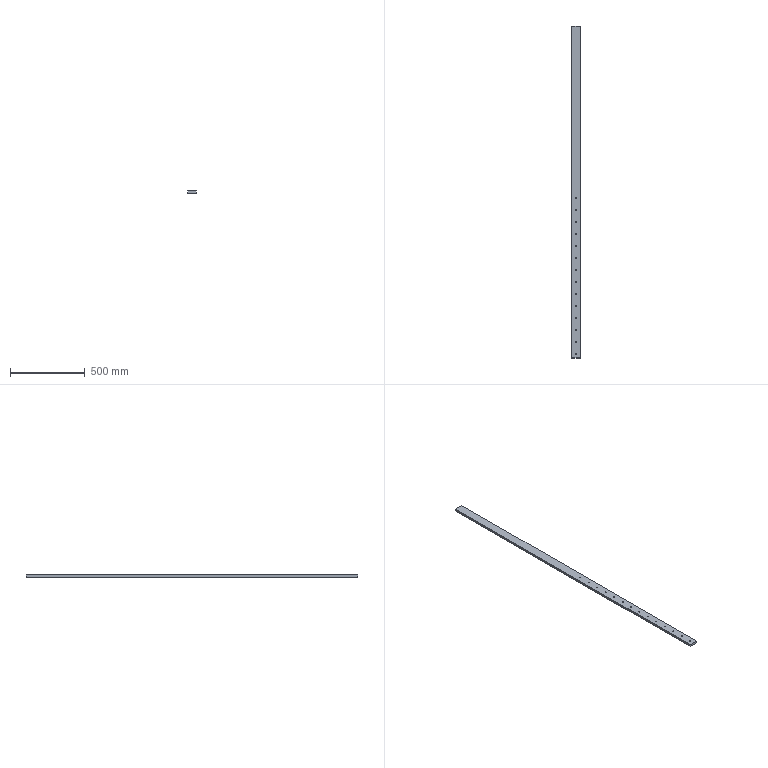Part | SolidWorks | features BaseBody 1 | 1 solid | 34 faces | box 60 x 2220 x 15 mm | volume 1990373 mm3 | cylinder 28 | plane 6 | commonest cylinder face diameters 6.8 x28
STEP:
#1=CARTESIAN_POINT('',(563.4,1142.,-1300.));
#2=VERTEX_POINT('',#1);
#3=CARTESIAN_POINT('',(556.6,1142.,-1300.));
#4=VERTEX_POINT('',#3);
#5=CARTESIAN_POINT('',(560.,1142.,-1300.));
#6=DIRECTION('',(0.,0.,-1.));
#7=DIRECTION('',(1.,0.,0.));
#8=AXIS2_PLACEMENT_3D('',#5,#6,#7);
#9=CIRCLE('',#8,3.4);
#10=EDGE_CURVE('',#2,#4,#9,.T.);
#11=ORIENTED_EDGE('',*,*,#10,.T.);
#12=CARTESIAN_POINT('',(556.6,1142.,-1285.));
#13=VERTEX_POINT('',#12);
#14=CARTESIAN_POINT('',(556.6,1142.,-1285.));
#15=DIRECTION('',(0.,0.,1.));
#16=VECTOR('',#15,1000.);
#17=LINE('',#14,#16);
#18=EDGE_CURVE('',#4,#13,#17,.T.);
#19=ORIENTED_EDGE('',*,*,#18,.T.);
#20=CARTESIAN_POINT('',(563.4,1142.,-1285.));
#21=VERTEX_POINT('',#20);
#22=CARTESIAN_POINT('',(560.,1142.,-1285.));
#23=DIRECTION('',(0.,0.,-1.));
#24=DIRECTION('',(1.,0.,0.));
#25=AXIS2_PLACEMENT_3D('',#22,#23,#24);
#26=CIRCLE('',#25,3.4);
#27=EDGE_CURVE('',#21,#13,#26,.T.);
#28=ORIENTED_EDGE('',*,*,#27,.F.);
#29=CARTESIAN_POINT('',(563.4,1142.,-1285.));
#30=DIRECTION('',(0.,0.,1.));
#31=VECTOR('',#30,1000.);
#32=LINE('',#29,#31);
#33=EDGE_CURVE('',#2,#21,#32,.T.);
#34=ORIENTED_EDGE('',*,*,#33,.F.);
#35=EDGE_LOOP('',(#11,#19,#28,#34));
#36=FACE_OUTER_BOUND('',#35,.T.);
#37=CARTESIAN_POINT('',(560.,1142.,-1285.));
#38=DIRECTION('',(0.,0.,1.));
#39=DIRECTION('',(1.,0.,0.));
#40=AXIS2_PLACEMENT_3D('',#37,#38,#39);
#41=CYLINDRICAL_SURFACE('',#40,3.4);
#42=ADVANCED_FACE('',(#36),#41,.F.);
#43=CARTESIAN_POINT('',(563.4,102.,-1300.));
#44=VERTEX_POINT('',#43);
#45=CARTESIAN_POINT('',(556.6,102.,-1300.));
#46=VERTEX_POINT('',#45);
#47=CARTESIAN_POINT('',(560.,102.,-1300.));
#48=DIRECTION('',(0.,0.,-1.));
#49=DIRECTION('',(1.,0.,0.));
#50=AXIS2_PLACEMENT_3D('',#47,#48,#49);
#51=CIRCLE('',#50,3.4);
#52=EDGE_CURVE('',#44,#46,#51,.T.);
#53=ORIENTED_EDGE('',*,*,#52,.T.);
#54=CARTESIAN_POINT('',(556.6,102.,-1285.));
#55=VERTEX_POINT('',#54);
#56=CARTESIAN_POINT('',(556.6,102.,-1285.));
#57=DIRECTION('',(0.,0.,1.));
#58=VECTOR('',#57,1000.);
#59=LINE('',#56,#58);
#60=EDGE_CURVE('',#46,#55,#59,.T.);
#61=ORIENTED_EDGE('',*,*,#60,.T.);
#62=CARTESIAN_POINT('',(563.4,102.,-1285.));
#63=VERTEX_POINT('',#62);
#64=CARTESIAN_POINT('',(560.,102.,-1285.));
#65=DIRECTION('',(0.,0.,-1.));
#66=DIRECTION('',(1.,0.,0.));
#67=AXIS2_PLACEMENT_3D('',#64,#65,#66);
#68=CIRCLE('',#67,3.4);
#69=EDGE_CURVE('',#63,#55,#68,.T.);
#70=ORIENTED_EDGE('',*,*,#69,.F.);
#71=CARTESIAN_POINT('',(563.4,102.,-1285.));
#72=DIRECTION('',(0.,0.,1.));
#73=VECTOR('',#72,1000.);
#74=LINE('',#71,#73);
#75=EDGE_CURVE('',#44,#63,#74,.T.);
#76=ORIENTED_EDGE('',*,*,#75,.F.);
#77=EDGE_LOOP('',(#53,#61,#70,#76));
#78=FACE_OUTER_BOUND('',#77,.T.);
#79=CARTESIAN_POINT('',(560.,102.,-1285.));
#80=DIRECTION('',(0.,0.,1.));
#81=DIRECTION('',(1.,0.,0.));
#82=AXIS2_PLACEMENT_3D('',#79,#80,#81);
#83=CYLINDRICAL_SURFACE('',#82,3.4);
#84=ADVANCED_FACE('',(#78),#83,.F.);
#85=CARTESIAN_POINT('',(563.4,182.,-1300.));
#86=VERTEX_POINT('',#85);
#87=CARTESIAN_POINT('',(556.6,182.,-1300.));
#88=VERTEX_POINT('',#87);
#89=CARTESIAN_POINT('',(560.,182.,-1300.));
#90=DIRECTION('',(0.,0.,-1.));
#91=DIRECTION('',(1.,0.,0.));
#92=AXIS2_PLACEMENT_3D('',#89,#90,#91);
#93=CIRCLE('',#92,3.4);
#94=EDGE_CURVE('',#86,#88,#93,.T.);
#95=ORIENTED_EDGE('',*,*,#94,.T.);
#96=CARTESIAN_POINT('',(556.6,182.,-1285.));
#97=VERTEX_POINT('',#96);
#98=CARTESIAN_POINT('',(556.6,182.,-1285.));
#99=DIRECTION('',(0.,0.,1.));
#100=VECTOR('',#99,1000.);
#101=LINE('',#98,#100);
#102=EDGE_CURVE('',#88,#97,#101,.T.);
#103=ORIENTED_EDGE('',*,*,#102,.T.);
#104=CARTESIAN_POINT('',(563.4,182.,-1285.));
#105=VERTEX_POINT('',#104);
#106=CARTESIAN_POINT('',(560.,182.,-1285.));
#107=DIRECTION('',(0.,0.,-1.));
#108=DIRECTION('',(1.,0.,0.));
#109=AXIS2_PLACEMENT_3D('',#106,#107,#108);
#110=CIRCLE('',#109,3.4);
#111=EDGE_CURVE('',#105,#97,#110,.T.);
#112=ORIENTED_EDGE('',*,*,#111,.F.);
#113=CARTESIAN_POINT('',(563.4,182.,-1285.));
#114=DIRECTION('',(0.,0.,1.));
#115=VECTOR('',#114,1000.);
#116=LINE('',#113,#115);
#117=EDGE_CURVE('',#86,#105,#116,.T.);
#118=ORIENTED_EDGE('',*,*,#117,.F.);
#119=EDGE_LOOP('',(#95,#103,#112,#118));
#120=FACE_OUTER_BOUND('',#119,.T.);
#121=CARTESIAN_POINT('',(560.,182.,-1285.));
#122=DIRECTION('',(0.,0.,1.));
#123=DIRECTION('',(1.,0.,0.));
#124=AXIS2_PLACEMENT_3D('',#121,#122,#123);
#125=CYLINDRICAL_SURFACE('',#124,3.4);
#126=ADVANCED_FACE('',(#120),#125,.F.);
#127=CARTESIAN_POINT('',(563.4,262.,-1300.));
#128=VERTEX_POINT('',#127);
#129=CARTESIAN_POINT('',(556.6,262.,-1300.));
#130=VERTEX_POINT('',#129);
#131=CARTESIAN_POINT('',(560.,262.,-1300.));
#132=DIRECTION('',(0.,0.,-1.));
#133=DIRECTION('',(1.,0.,0.));
#134=AXIS2_PLACEMENT_3D('',#131,#132,#133);
#135=CIRCLE('',#134,3.4);
#136=EDGE_CURVE('',#128,#130,#135,.T.);
#137=ORIENTED_EDGE('',*,*,#136,.T.);
#138=CARTESIAN_POINT('',(556.6,262.,-1285.));
#139=VERTEX_POINT('',#138);
#140=CARTESIAN_POINT('',(556.6,262.,-1285.));
#141=DIRECTION('',(0.,0.,1.));
#142=VECTOR('',#141,1000.);
#143=LINE('',#140,#142);
#144=EDGE_CURVE('',#130,#139,#143,.T.);
#145=ORIENTED_EDGE('',*,*,#144,.T.);
#146=CARTESIAN_POINT('',(563.4,262.,-1285.));
#147=VERTEX_POINT('',#146);
#148=CARTESIAN_POINT('',(560.,262.,-1285.));
#149=DIRECTION('',(0.,0.,-1.));
#150=DIRECTION('',(1.,0.,0.));
#151=AXIS2_PLACEMENT_3D('',#148,#149,#150);
#152=CIRCLE('',#151,3.4);
#153=EDGE_CURVE('',#147,#139,#152,.T.);
#154=ORIENTED_EDGE('',*,*,#153,.F.);
#155=CARTESIAN_POINT('',(563.4,262.,-1285.));
#156=DIRECTION('',(0.,0.,1.));
#157=VECTOR('',#156,1000.);
#158=LINE('',#155,#157);
#159=EDGE_CURVE('',#128,#147,#158,.T.);
#160=ORIENTED_EDGE('',*,*,#159,.F.);
#161=EDGE_LOOP('',(#137,#145,#154,#160));
#162=FACE_OUTER_BOUND('',#161,.T.);
#163=CARTESIAN_POINT('',(560.,262.,-1285.));
#164=DIRECTION('',(0.,0.,1.));
#165=DIRECTION('',(1.,0.,0.));
#166=AXIS2_PLACEMENT_3D('',#163,#164,#165);
#167=CYLINDRICAL_SURFACE('',#166,3.4);
#168=ADVANCED_FACE('',(#162),#167,.F.);
#169=CARTESIAN_POINT('',(563.4,342.,-1300.));
#170=VERTEX_POINT('',#169);
#171=CARTESIAN_POINT('',(556.6,342.,-1300.));
#172=VERTEX_POINT('',#171);
#173=CARTESIAN_POINT('',(560.,342.,-1300.));
#174=DIRECTION('',(0.,0.,-1.));
#175=DIRECTION('',(1.,0.,0.));
#176=AXIS2_PLACEMENT_3D('',#173,#174,#175);
#177=CIRCLE('',#176,3.4);
#178=EDGE_CURVE('',#170,#172,#177,.T.);
#179=ORIENTED_EDGE('',*,*,#178,.T.);
#180=CARTESIAN_POINT('',(556.6,342.,-1285.));
#181=VERTEX_POINT('',#180);
#182=CARTESIAN_POINT('',(556.6,342.,-1285.));
#183=DIRECTION('',(0.,0.,1.));
#184=VECTOR('',#183,1000.);
#185=LINE('',#182,#184);
#186=EDGE_CURVE('',#172,#181,#185,.T.);
#187=ORIENTED_EDGE('',*,*,#186,.T.);
#188=CARTESIAN_POINT('',(563.4,342.,-1285.));
#189=VERTEX_POINT('',#188);
#190=CARTESIAN_POINT('',(560.,342.,-1285.));
#191=DIRECTION('',(0.,0.,-1.));
#192=DIRECTION('',(1.,0.,0.));
#193=AXIS2_PLACEMENT_3D('',#190,#191,#192);
#194=CIRCLE('',#193,3.4);
#195=EDGE_CURVE('',#189,#181,#194,.T.);
#196=ORIENTED_EDGE('',*,*,#195,.F.);
#197=CARTESIAN_POINT('',(563.4,342.,-1285.));
#198=DIRECTION('',(0.,0.,1.));
#199=VECTOR('',#198,1000.);
#200=LINE('',#197,#199);
#201=EDGE_CURVE('',#170,#189,#200,.T.);
#202=ORIENTED_EDGE('',*,*,#201,.F.);
#203=EDGE_LOOP('',(#179,#187,#196,#202));
#204=FACE_OUTER_BOUND('',#203,.T.);
#205=CARTESIAN_POINT('',(560.,342.,-1285.));
#206=DIRECTION('',(0.,0.,1.));
#207=DIRECTION('',(1.,0.,0.));
#208=AXIS2_PLACEMENT_3D('',#205,#206,#207);
#209=CYLINDRICAL_SURFACE('',#208,3.4);
#210=ADVANCED_FACE('',(#204),#209,.F.);
#211=CARTESIAN_POINT('',(563.4,422.,-1300.));
#212=VERTEX_POINT('',#211);
#213=CARTESIAN_POINT('',(556.6,422.,-1300.));
#214=VERTEX_POINT('',#213);
#215=CARTESIAN_POINT('',(560.,422.,-1300.));
#216=DIRECTION('',(0.,0.,-1.));
#217=DIRECTION('',(1.,0.,0.));
#218=AXIS2_PLACEMENT_3D('',#215,#216,#217);
#219=CIRCLE('',#218,3.4);
#220=EDGE_CURVE('',#212,#214,#219,.T.);
#221=ORIENTED_EDGE('',*,*,#220,.T.);
#222=CARTESIAN_POINT('',(556.6,422.,-1285.));
#223=VERTEX_POINT('',#222);
#224=CARTESIAN_POINT('',(556.6,422.,-1285.));
#225=DIRECTION('',(0.,0.,1.));
#226=VECTOR('',#225,1000.);
#227=LINE('',#224,#226);
#228=EDGE_CURVE('',#214,#223,#227,.T.);
#229=ORIENTED_EDGE('',*,*,#228,.T.);
#230=CARTESIAN_POINT('',(563.4,422.,-1285.));
#231=VERTEX_POINT('',#230);
#232=CARTESIAN_POINT('',(560.,422.,-1285.));
#233=DIRECTION('',(0.,0.,-1.));
#234=DIRECTION('',(1.,0.,0.));
#235=AXIS2_PLACEMENT_3D('',#232,#233,#234);
#236=CIRCLE('',#235,3.4);
#237=EDGE_CURVE('',#231,#223,#236,.T.);
#238=ORIENTED_EDGE('',*,*,#237,.F.);
#239=CARTESIAN_POINT('',(563.4,422.,-1285.));
#240=DIRECTION('',(0.,0.,1.));
#241=VECTOR('',#240,1000.);
#242=LINE('',#239,#241);
#243=EDGE_CURVE('',#212,#231,#242,.T.);
#244=ORIENTED_EDGE('',*,*,#243,.F.);
#245=EDGE_LOOP('',(#221,#229,#238,#244));
#246=FACE_OUTER_BOUND('',#245,.T.);
#247=CARTESIAN_POINT('',(560.,422.,-1285.));
#248=DIRECTION('',(0.,0.,1.));
#249=DIRECTION('',(1.,0.,0.));
#250=AXIS2_PLACEMENT_3D('',#247,#248,#249);
#251=CYLINDRICAL_SURFACE('',#250,3.4);
#252=ADVANCED_FACE('',(#246),#251,.F.);
#253=CARTESIAN_POINT('',(563.4,502.,-1300.));
#254=VERTEX_POINT('',#253);
#255=CARTESIAN_POINT('',(556.6,502.,-1300.));
#256=VERTEX_POINT('',#255);
#257=CARTESIAN_POINT('',(560.,502.,-1300.));
#258=DIRECTION('',(0.,0.,-1.));
#259=DIRECTION('',(1.,0.,0.));
#260=AXIS2_PLACEMENT_3D('',#257,#258,#259);
#261=CIRCLE('',#260,3.4);
#262=EDGE_CURVE('',#254,#256,#261,.T.);
#263=ORIENTED_EDGE('',*,*,#262,.T.);
#264=CARTESIAN_POINT('',(556.6,502.,-1285.));
#265=VERTEX_POINT('',#264);
#266=CARTESIAN_POINT('',(556.6,502.,-1285.));
#267=DIRECTION('',(0.,0.,1.));
#268=VECTOR('',#267,1000.);
#269=LINE('',#266,#268);
#270=EDGE_CURVE('',#256,#265,#269,.T.);
#271=ORIENTED_EDGE('',*,*,#270,.T.);
#272=CARTESIAN_POINT('',(563.4,502.,-1285.));
#273=VERTEX_POINT('',#272);
#274=CARTESIAN_POINT('',(560.,502.,-1285.));
#275=DIRECTION('',(0.,0.,-1.));
#276=DIRECTION('',(1.,0.,0.));
#277=AXIS2_PLACEMENT_3D('',#274,#275,#276);
#278=CIRCLE('',#277,3.4);
#279=EDGE_CURVE('',#273,#265,#278,.T.);
#280=ORIENTED_EDGE('',*,*,#279,.F.);
#281=CARTESIAN_POINT('',(563.4,502.,-1285.));
#282=DIRECTION('',(0.,0.,1.));
#283=VECTOR('',#282,1000.);
#284=LINE('',#281,#283);
#285=EDGE_CURVE('',#254,#273,#284,.T.);
#286=ORIENTED_EDGE('',*,*,#285,.F.);
#287=EDGE_LOOP('',(#263,#271,#280,#286));
#288=FACE_OUTER_BOUND('',#287,.T.);
#289=CARTESIAN_POINT('',(560.,502.,-1285.));
#290=DIRECTION('',(0.,0.,1.));
#291=DIRECTION('',(1.,0.,0.));
#292=AXIS2_PLACEMENT_3D('',#289,#290,#291);
#293=CYLINDRICAL_SURFACE('',#292,3.4);
#294=ADVANCED_FACE('',(#288),#293,.F.);
#295=CARTESIAN_POINT('',(563.4,582.,-1300.));
#296=VERTEX_POINT('',#295);
#297=CARTESIAN_POINT('',(556.6,582.,-1300.));
#298=VERTEX_POINT('',#297);
#299=CARTESIAN_POINT('',(560.,582.,-1300.));
#300=DIRECTION('',(0.,0.,-1.));
#301=DIRECTION('',(1.,0.,0.));
#302=AXIS2_PLACEMENT_3D('',#299,#300,#301);
#303=CIRCLE('',#302,3.4);
#304=EDGE_CURVE('',#296,#298,#303,.T.);
#305=ORIENTED_EDGE('',*,*,#304,.T.);
#306=CARTESIAN_POINT('',(556.6,582.,-1285.));
#307=VERTEX_POINT('',#306);
#308=CARTESIAN_POINT('',(556.6,582.,-1285.));
#309=DIRECTION('',(0.,0.,1.));
#310=VECTOR('',#309,1000.);
#311=LINE('',#308,#310);
#312=EDGE_CURVE('',#298,#307,#311,.T.);
#313=ORIENTED_EDGE('',*,*,#312,.T.);
#314=CARTESIAN_POINT('',(563.4,582.,-1285.));
#315=VERTEX_POINT('',#314);
#316=CARTESIAN_POINT('',(560.,582.,-1285.));
#317=DIRECTION('',(0.,0.,-1.));
#318=DIRECTION('',(1.,0.,0.));
#319=AXIS2_PLACEMENT_3D('',#316,#317,#318);
#320=CIRCLE('',#319,3.4);
#321=EDGE_CURVE('',#315,#307,#320,.T.);
#322=ORIENTED_EDGE('',*,*,#321,.F.);
#323=CARTESIAN_POINT('',(563.4,582.,-1285.));
#324=DIRECTION('',(0.,0.,1.));
#325=VECTOR('',#324,1000.);
#326=LINE('',#323,#325);
#327=EDGE_CURVE('',#296,#315,#326,.T.);
#328=ORIENTED_EDGE('',*,*,#327,.F.);
#329=EDGE_LOOP('',(#305,#313,#322,#328));
#330=FACE_OUTER_BOUND('',#329,.T.);
#331=CARTESIAN_POINT('',(560.,582.,-1285.));
#332=DIRECTION('',(0.,0.,1.));
#333=DIRECTION('',(1.,0.,0.));
#334=AXIS2_PLACEMENT_3D('',#331,#332,#333);
#335=CYLINDRICAL_SURFACE('',#334,3.4);
#336=ADVANCED_FACE('',(#330),#335,.F.);
#337=CARTESIAN_POINT('',(563.4,662.,-1300.));
#338=VERTEX_POINT('',#337);
#339=CARTESIAN_POINT('',(556.6,662.,-1300.));
#340=VERTEX_POINT('',#339);
#341=CARTESIAN_POINT('',(560.,662.,-1300.));
#342=DIRECTION('',(0.,0.,-1.));
#343=DIRECTION('',(1.,0.,0.));
#344=AXIS2_PLACEMENT_3D('',#341,#342,#343);
#345=CIRCLE('',#344,3.4);
#346=EDGE_CURVE('',#338,#340,#345,.T.);
#347=ORIENTED_EDGE('',*,*,#346,.T.);
#348=CARTESIAN_POINT('',(556.6,662.,-1285.));
#349=VERTEX_POINT('',#348);
#350=CARTESIAN_POINT('',(556.6,662.,-1285.));
#351=DIRECTION('',(0.,0.,1.));
#352=VECTOR('',#351,1000.);
#353=LINE('',#350,#352);
#354=EDGE_CURVE('',#340,#349,#353,.T.);
#355=ORIENTED_EDGE('',*,*,#354,.T.);
#356=CARTESIAN_POINT('',(563.4,662.,-1285.));
#357=VERTEX_POINT('',#356);
#358=CARTESIAN_POINT('',(560.,662.,-1285.));
#359=DIRECTION('',(0.,0.,-1.));
#360=DIRECTION('',(1.,0.,0.));
#361=AXIS2_PLACEMENT_3D('',#358,#359,#360);
#362=CIRCLE('',#361,3.4);
#363=EDGE_CURVE('',#357,#349,#362,.T.);
#364=ORIENTED_EDGE('',*,*,#363,.F.);
#365=CARTESIAN_POINT('',(563.4,662.,-1285.));
#366=DIRECTION('',(0.,0.,1.));
#367=VECTOR('',#366,1000.);
#368=LINE('',#365,#367);
#369=EDGE_CURVE('',#338,#357,#368,.T.);
#370=ORIENTED_EDGE('',*,*,#369,.F.);
#371=EDGE_LOOP('',(#347,#355,#364,#370));
#372=FACE_OUTER_BOUND('',#371,.T.);
#373=CARTESIAN_POINT('',(560.,662.,-1285.));
#374=DIRECTION('',(0.,0.,1.));
#375=DIRECTION('',(1.,0.,0.));
#376=AXIS2_PLACEMENT_3D('',#373,#374,#375);
#377=CYLINDRICAL_SURFACE('',#376,3.4);
#378=ADVANCED_FACE('',(#372),#377,.F.);
#379=CARTESIAN_POINT('',(563.4,742.,-1300.));
#380=VERTEX_POINT('',#379);
#381=CARTESIAN_POINT('',(556.6,742.,-1300.));
#382=VERTEX_POINT('',#381);
#383=CARTESIAN_POINT('',(560.,742.,-1300.));
#384=DIRECTION('',(0.,0.,-1.));
#385=DIRECTION('',(1.,0.,0.));
#386=AXIS2_PLACEMENT_3D('',#383,#384,#385);
#387=CIRCLE('',#386,3.4);
#388=EDGE_CURVE('',#380,#382,#387,.T.);
#389=ORIENTED_EDGE('',*,*,#388,.T.);
#390=CARTESIAN_POINT('',(556.6,742.,-1285.));
#391=VERTEX_POINT('',#390);
#392=CARTESIAN_POINT('',(556.6,742.,-1285.));
#393=DIRECTION('',(0.,0.,1.));
#394=VECTOR('',#393,1000.);
#395=LINE('',#392,#394);
#396=EDGE_CURVE('',#382,#391,#395,.T.);
#397=ORIENTED_EDGE('',*,*,#396,.T.);
#398=CARTESIAN_POINT('',(563.4,742.,-1285.));
#399=VERTEX_POINT('',#398);
#400=CARTESIAN_POINT('',(560.,742.,-1285.));
#401=DIRECTION('',(0.,0.,-1.));
#402=DIRECTION('',(1.,0.,0.));
#403=AXIS2_PLACEMENT_3D('',#400,#401,#402);
#404=CIRCLE('',#403,3.4);
#405=EDGE_CURVE('',#399,#391,#404,.T.);
#406=ORIENTED_EDGE('',*,*,#405,.F.);
#407=CARTESIAN_POINT('',(563.4,742.,-1285.));
#408=DIRECTION('',(0.,0.,1.));
#409=VECTOR('',#408,1000.);
#410=LINE('',#407,#409);
#411=EDGE_CURVE('',#380,#399,#410,.T.);
#412=ORIENTED_EDGE('',*,*,#411,.F.);
#413=EDGE_LOOP('',(#389,#397,#406,#412));
#414=FACE_OUTER_BOUND('',#413,.T.);
#415=CARTESIAN_POINT('',(560.,742.,-1285.));
#416=DIRECTION('',(0.,0.,1.));
#417=DIRECTION('',(1.,0.,0.));
#418=AXIS2_PLACEMENT_3D('',#415,#416,#417);
#419=CYLINDRICAL_SURFACE('',#418,3.4);
#420=ADVANCED_FACE('',(#414),#419,.F.);
#421=CARTESIAN_POINT('',(563.4,822.,-1300.));
#422=VERTEX_POINT('',#421);
#423=CARTESIAN_POINT('',(556.6,822.,-1300.));
#424=VERTEX_POINT('',#423);
#425=CARTESIAN_POINT('',(560.,822.,-1300.));
#426=DIRECTION('',(0.,0.,-1.));
#427=DIRECTION('',(1.,0.,0.));
#428=AXIS2_PLACEMENT_3D('',#425,#426,#427);
#429=CIRCLE('',#428,3.4);
#430=EDGE_CURVE('',#422,#424,#429,.T.);
#431=ORIENTED_EDGE('',*,*,#430,.T.);
#432=CARTESIAN_POINT('',(556.6,822.,-1285.));
#433=VERTEX_POINT('',#432);
#434=CARTESIAN_POINT('',(556.6,822.,-1285.));
#435=DIRECTION('',(0.,0.,1.));
#436=VECTOR('',#435,1000.);
#437=LINE('',#434,#436);
#438=EDGE_CURVE('',#424,#433,#437,.T.);
#439=ORIENTED_EDGE('',*,*,#438,.T.);
#440=CARTESIAN_POINT('',(563.4,822.,-1285.));
#441=VERTEX_POINT('',#440);
#442=CARTESIAN_POINT('',(560.,822.,-1285.));
#443=DIRECTION('',(0.,0.,-1.));
#444=DIRECTION('',(1.,0.,0.));
#445=AXIS2_PLACEMENT_3D('',#442,#443,#444);
#446=CIRCLE('',#445,3.4);
#447=EDGE_CURVE('',#441,#433,#446,.T.);
#448=ORIENTED_EDGE('',*,*,#447,.F.);
#449=CARTESIAN_POINT('',(563.4,822.,-1285.));
#450=DIRECTION('',(0.,0.,1.));
#451=VECTOR('',#450,1000.);
#452=LINE('',#449,#451);
#453=EDGE_CURVE('',#422,#441,#452,.T.);
#454=ORIENTED_EDGE('',*,*,#453,.F.);
#455=EDGE_LOOP('',(#431,#439,#448,#454));
#456=FACE_OUTER_BOUND('',#455,.T.);
#457=CARTESIAN_POINT('',(560.,822.,-1285.));
#458=DIRECTION('',(0.,0.,1.));
#459=DIRECTION('',(1.,0.,0.));
#460=AXIS2_PLACEMENT_3D('',#457,#458,#459);
#461=CYLINDRICAL_SURFACE('',#460,3.4);
#462=ADVANCED_FACE('',(#456),#461,.F.);
#463=CARTESIAN_POINT('',(563.4,902.,-1300.));
#464=VERTEX_POINT('',#463);
#465=CARTESIAN_POINT('',(556.6,902.,-1300.));
#466=VERTEX_POINT('',#465);
#467=CARTESIAN_POINT('',(560.,902.,-1300.));
#468=DIRECTION('',(0.,0.,-1.));
#469=DIRECTION('',(1.,0.,0.));
#470=AXIS2_PLACEMENT_3D('',#467,#468,#469);
#471=CIRCLE('',#470,3.4);
#472=EDGE_CURVE('',#464,#466,#471,.T.);
#473=ORIENTED_EDGE('',*,*,#472,.T.);
#474=CARTESIAN_POINT('',(556.6,902.,-1285.));
#475=VERTEX_POINT('',#474);
#476=CARTESIAN_POINT('',(556.6,902.,-1285.));
#477=DIRECTION('',(0.,0.,1.));
#478=VECTOR('',#477,1000.);
#479=LINE('',#476,#478);
#480=EDGE_CURVE('',#466,#475,#479,.T.);
#481=ORIENTED_EDGE('',*,*,#480,.T.);
#482=CARTESIAN_POINT('',(563.4,902.,-1285.));
#483=VERTEX_POINT('',#482);
#484=CARTESIAN_POINT('',(560.,902.,-1285.));
#485=DIRECTION('',(0.,0.,-1.));
#486=DIRECTION('',(1.,0.,0.));
#487=AXIS2_PLACEMENT_3D('',#484,#485,#486);
#488=CIRCLE('',#487,3.4);
#489=EDGE_CURVE('',#483,#475,#488,.T.);
#490=ORIENTED_EDGE('',*,*,#489,.F.);
#491=CARTESIAN_POINT('',(563.4,902.,-1285.));
#492=DIRECTION('',(0.,0.,1.));
#493=VECTOR('',#492,1000.);
#494=LINE('',#491,#493);
#495=EDGE_CURVE('',#464,#483,#494,.T.);
#496=ORIENTED_EDGE('',*,*,#495,.F.);
#497=EDGE_LOOP('',(#473,#481,#490,#496));
#498=FACE_OUTER_BOUND('',#497,.T.);
#499=CARTESIAN_POINT('',(560.,902.,-1285.));
#500=DIRECTION('',(0.,0.,1.));
#501=DIRECTION('',(1.,0.,0.));
#502=AXIS2_PLACEMENT_3D('',#499,#500,#501);
#503=CYLINDRICAL_SURFACE('',#502,3.4);
#504=ADVANCED_FACE('',(#498),#503,.F.);
#505=CARTESIAN_POINT('',(563.4,982.,-1300.));
#506=VERTEX_POINT('',#505);
#507=CARTESIAN_POINT('',(556.6,982.,-1300.));
#508=VERTEX_POINT('',#507);
#509=CARTESIAN_POINT('',(560.,982.,-1300.));
#510=DIRECTION('',(0.,0.,-1.));
#511=DIRECTION('',(1.,0.,0.));
#512=AXIS2_PLACEMENT_3D('',#509,#510,#511);
#513=CIRCLE('',#512,3.4);
#514=EDGE_CURVE('',#506,#508,#513,.T.);
#515=ORIENTED_EDGE('',*,*,#514,.T.);
#516=CARTESIAN_POINT('',(556.6,982.,-1285.));
#517=VERTEX_POINT('',#516);
#518=CARTESIAN_POINT('',(556.6,982.,-1285.));
#519=DIRECTION('',(0.,0.,1.));
#520=VECTOR('',#519,1000.);
#521=LINE('',#518,#520);
#522=EDGE_CURVE('',#508,#517,#521,.T.);
#523=ORIENTED_EDGE('',*,*,#522,.T.);
#524=CARTESIAN_POINT('',(563.4,982.,-1285.));
#525=VERTEX_POINT('',#524);
#526=CARTESIAN_POINT('',(560.,982.,-1285.));
#527=DIRECTION('',(0.,0.,-1.));
#528=DIRECTION('',(1.,0.,0.));
#529=AXIS2_PLACEMENT_3D('',#526,#527,#528);
#530=CIRCLE('',#529,3.4);
#531=EDGE_CURVE('',#525,#517,#530,.T.);
#532=ORIENTED_EDGE('',*,*,#531,.F.);
#533=CARTESIAN_POINT('',(563.4,982.,-1285.));
#534=DIRECTION('',(0.,0.,1.));
#535=VECTOR('',#534,1000.);
#536=LINE('',#533,#535);
#537=EDGE_CURVE('',#506,#525,#536,.T.);
#538=ORIENTED_EDGE('',*,*,#537,.F.);
#539=EDGE_LOOP('',(#515,#523,#532,#538));
#540=FACE_OUTER_BOUND('',#539,.T.);
#541=CARTESIAN_POINT('',(560.,982.,-1285.));
#542=DIRECTION('',(0.,0.,1.));
#543=DIRECTION('',(1.,0.,0.));
#544=AXIS2_PLACEMENT_3D('',#541,#542,#543);
#545=CYLINDRICAL_SURFACE('',#544,3.4);
#546=ADVANCED_FACE('',(#540),#545,.F.);
#547=CARTESIAN_POINT('',(563.4,1062.,-1300.));
#548=VERTEX_POINT('',#547);
#549=CARTESIAN_POINT('',(556.6,1062.,-1300.));
#550=VERTEX_POINT('',#549);
#551=CARTESIAN_POINT('',(560.,1062.,-1300.));
#552=DIRECTION('',(0.,0.,-1.));
#553=DIRECTION('',(1.,0.,0.));
#554=AXIS2_PLACEMENT_3D('',#551,#552,#553);
#555=CIRCLE('',#554,3.4);
#556=EDGE_CURVE('',#548,#550,#555,.T.);
#557=ORIENTED_EDGE('',*,*,#556,.T.);
#558=CARTESIAN_POINT('',(556.6,1062.,-1285.));
#559=VERTEX_POINT('',#558);
#560=CARTESIAN_POINT('',(556.6,1062.,-1285.));
#561=DIRECTION('',(0.,0.,1.));
#562=VECTOR('',#561,1000.);
#563=LINE('',#560,#562);
#564=EDGE_CURVE('',#550,#559,#563,.T.);
#565=ORIENTED_EDGE('',*,*,#564,.T.);
#566=CARTESIAN_POINT('',(563.4,1062.,-1285.));
#567=VERTEX_POINT('',#566);
#568=CARTESIAN_POINT('',(560.,1062.,-1285.));
#569=DIRECTION('',(0.,0.,-1.));
#570=DIRECTION('',(1.,0.,0.));
#571=AXIS2_PLACEMENT_3D('',#568,#569,#570);
#572=CIRCLE('',#571,3.4);
#573=EDGE_CURVE('',#567,#559,#572,.T.);
#574=ORIENTED_EDGE('',*,*,#573,.F.);
#575=CARTESIAN_POINT('',(563.4,1062.,-1285.));
#576=DIRECTION('',(0.,0.,1.));
#577=VECTOR('',#576,1000.);
#578=LINE('',#575,#577);
#579=EDGE_CURVE('',#548,#567,#578,.T.);
#580=ORIENTED_EDGE('',*,*,#579,.F.);
#581=EDGE_LOOP('',(#557,#565,#574,#580));
#582=FACE_OUTER_BOUND('',#581,.T.);
#583=CARTESIAN_POINT('',(560.,1062.,-1285.));
#584=DIRECTION('',(0.,0.,1.));
#585=DIRECTION('',(1.,0.,0.));
#586=AXIS2_PLACEMENT_3D('',#583,#584,#585);
#587=CYLINDRICAL_SURFACE('',#586,3.4);
#588=ADVANCED_FACE('',(#582),#587,.F.);
#589=ORIENTED_EDGE('',*,*,#10,.F.);
#590=CARTESIAN_POINT('',(560.,1142.,-1300.));
#591=DIRECTION('',(0.,0.,-1.));
#592=DIRECTION('',(1.,0.,0.));
#593=AXIS2_PLACEMENT_3D('',#590,#591,#592);
#594=CIRCLE('',#593,3.4);
#595=EDGE_CURVE('',#4,#2,#594,.T.);
#596=ORIENTED_EDGE('',*,*,#595,.F.);
#597=EDGE_LOOP('',(#589,#596));
#598=FACE_BOUND('',#597,.T.);
#599=ORIENTED_EDGE('',*,*,#52,.F.);
#600=CARTESIAN_POINT('',(560.,102.,-1300.));
#601=DIRECTION('',(0.,0.,-1.));
#602=DIRECTION('',(1.,0.,0.));
#603=AXIS2_PLACEMENT_3D('',#600,#601,#602);
#604=CIRCLE('',#603,3.4);
#605=EDGE_CURVE('',#46,#44,#604,.T.);
#606=ORIENTED_EDGE('',*,*,#605,.F.);
#607=EDGE_LOOP('',(#599,#606));
#608=FACE_BOUND('',#607,.T.);
#609=ORIENTED_EDGE('',*,*,#94,.F.);
#610=CARTESIAN_POINT('',(560.,182.,-1300.));
#611=DIRECTION('',(0.,0.,-1.));
#612=DIRECTION('',(1.,0.,0.));
#613=AXIS2_PLACEMENT_3D('',#610,#611,#612);
#614=CIRCLE('',#613,3.4);
#615=EDGE_CURVE('',#88,#86,#614,.T.);
#616=ORIENTED_EDGE('',*,*,#615,.F.);
#617=EDGE_LOOP('',(#609,#616));
#618=FACE_BOUND('',#617,.T.);
#619=ORIENTED_EDGE('',*,*,#136,.F.);
#620=CARTESIAN_POINT('',(560.,262.,-1300.));
#621=DIRECTION('',(0.,0.,-1.));
#622=DIRECTION('',(1.,0.,0.));
#623=AXIS2_PLACEMENT_3D('',#620,#621,#622);
#624=CIRCLE('',#623,3.4);
#625=EDGE_CURVE('',#130,#128,#624,.T.);
#626=ORIENTED_EDGE('',*,*,#625,.F.);
#627=EDGE_LOOP('',(#619,#626));
#628=FACE_BOUND('',#627,.T.);
#629=ORIENTED_EDGE('',*,*,#178,.F.);
#630=CARTESIAN_POINT('',(560.,342.,-1300.));
#631=DIRECTION('',(0.,0.,-1.));
#632=DIRECTION('',(1.,0.,0.));
#633=AXIS2_PLACEMENT_3D('',#630,#631,#632);
#634=CIRCLE('',#633,3.4);
#635=EDGE_CURVE('',#172,#170,#634,.T.);
#636=ORIENTED_EDGE('',*,*,#635,.F.);
#637=EDGE_LOOP('',(#629,#636));
#638=FACE_BOUND('',#637,.T.);
#639=ORIENTED_EDGE('',*,*,#220,.F.);
#640=CARTESIAN_POINT('',(560.,422.,-1300.));
#641=DIRECTION('',(0.,0.,-1.));
#642=DIRECTION('',(1.,0.,0.));
#643=AXIS2_PLACEMENT_3D('',#640,#641,#642);
#644=CIRCLE('',#643,3.4);
#645=EDGE_CURVE('',#214,#212,#644,.T.);
#646=ORIENTED_EDGE('',*,*,#645,.F.);
#647=EDGE_LOOP('',(#639,#646));
#648=FACE_BOUND('',#647,.T.);
#649=ORIENTED_EDGE('',*,*,#262,.F.);
#650=CARTESIAN_POINT('',(560.,502.,-1300.));
#651=DIRECTION('',(0.,0.,-1.));
#652=DIRECTION('',(1.,0.,0.));
#653=AXIS2_PLACEMENT_3D('',#650,#651,#652);
#654=CIRCLE('',#653,3.4);
#655=EDGE_CURVE('',#256,#254,#654,.T.);
#656=ORIENTED_EDGE('',*,*,#655,.F.);
#657=EDGE_LOOP('',(#649,#656));
#658=FACE_BOUND('',#657,.T.);
#659=ORIENTED_EDGE('',*,*,#304,.F.);
#660=CARTESIAN_POINT('',(560.,582.,-1300.));
#661=DIRECTION('',(0.,0.,-1.));
#662=DIRECTION('',(1.,0.,0.));
#663=AXIS2_PLACEMENT_3D('',#660,#661,#662);
#664=CIRCLE('',#663,3.4);
#665=EDGE_CURVE('',#298,#296,#664,.T.);
#666=ORIENTED_EDGE('',*,*,#665,.F.);
#667=EDGE_LOOP('',(#659,#666));
#668=FACE_BOUND('',#667,.T.);
#669=ORIENTED_EDGE('',*,*,#346,.F.);
#670=CARTESIAN_POINT('',(560.,662.,-1300.));
#671=DIRECTION('',(0.,0.,-1.));
#672=DIRECTION('',(1.,0.,0.));
#673=AXIS2_PLACEMENT_3D('',#670,#671,#672);
#674=CIRCLE('',#673,3.4);
#675=EDGE_CURVE('',#340,#338,#674,.T.);
#676=ORIENTED_EDGE('',*,*,#675,.F.);
#677=EDGE_LOOP('',(#669,#676));
#678=FACE_BOUND('',#677,.T.);
#679=ORIENTED_EDGE('',*,*,#388,.F.);
#680=CARTESIAN_POINT('',(560.,742.,-1300.));
#681=DIRECTION('',(0.,0.,-1.));
#682=DIRECTION('',(1.,0.,0.));
#683=AXIS2_PLACEMENT_3D('',#680,#681,#682);
#684=CIRCLE('',#683,3.4);
#685=EDGE_CURVE('',#382,#380,#684,.T.);
#686=ORIENTED_EDGE('',*,*,#685,.F.);
#687=EDGE_LOOP('',(#679,#686));
#688=FACE_BOUND('',#687,.T.);
#689=ORIENTED_EDGE('',*,*,#430,.F.);
#690=CARTESIAN_POINT('',(560.,822.,-1300.));
#691=DIRECTION('',(0.,0.,-1.));
#692=DIRECTION('',(1.,0.,0.));
#693=AXIS2_PLACEMENT_3D('',#690,#691,#692);
#694=CIRCLE('',#693,3.4);
#695=EDGE_CURVE('',#424,#422,#694,.T.);
#696=ORIENTED_EDGE('',*,*,#695,.F.);
#697=EDGE_LOOP('',(#689,#696));
#698=FACE_BOUND('',#697,.T.);
#699=ORIENTED_EDGE('',*,*,#472,.F.);
#700=CARTESIAN_POINT('',(560.,902.,-1300.));
#701=DIRECTION('',(0.,0.,-1.));
#702=DIRECTION('',(1.,0.,0.));
#703=AXIS2_PLACEMENT_3D('',#700,#701,#702);
#704=CIRCLE('',#703,3.4);
#705=EDGE_CURVE('',#466,#464,#704,.T.);
#706=ORIENTED_EDGE('',*,*,#705,.F.);
#707=EDGE_LOOP('',(#699,#706));
#708=FACE_BOUND('',#707,.T.);
#709=ORIENTED_EDGE('',*,*,#514,.F.);
#710=CARTESIAN_POINT('',(560.,982.,-1300.));
#711=DIRECTION('',(0.,0.,-1.));
#712=DIRECTION('',(1.,0.,0.));
#713=AXIS2_PLACEMENT_3D('',#710,#711,#712);
#714=CIRCLE('',#713,3.4);
#715=EDGE_CURVE('',#508,#506,#714,.T.);
#716=ORIENTED_EDGE('',*,*,#715,.F.);
#717=EDGE_LOOP('',(#709,#716));
#718=FACE_BOUND('',#717,.T.);
#719=ORIENTED_EDGE('',*,*,#556,.F.);
#720=CARTESIAN_POINT('',(560.,1062.,-1300.));
#721=DIRECTION('',(0.,0.,-1.));
#722=DIRECTION('',(1.,0.,0.));
#723=AXIS2_PLACEMENT_3D('',#720,#721,#722);
#724=CIRCLE('',#723,3.4);
#725=EDGE_CURVE('',#550,#548,#724,.T.);
#726=ORIENTED_EDGE('',*,*,#725,.F.);
#727=EDGE_LOOP('',(#719,#726));
#728=FACE_BOUND('',#727,.T.);
#729=CARTESIAN_POINT('',(590.,2292.,-1300.));
#730=VERTEX_POINT('',#729);
#731=CARTESIAN_POINT('',(530.,2292.,-1300.));
#732=VERTEX_POINT('',#731);
#733=CARTESIAN_POINT('',(530.,2292.,-1300.));
#734=DIRECTION('',(-1.,0.,0.));
#735=VECTOR('',#734,1000.);
#736=LINE('',#733,#735);
#737=EDGE_CURVE('',#730,#732,#736,.T.);
#738=ORIENTED_EDGE('',*,*,#737,.F.);
#739=CARTESIAN_POINT('',(590.,72.,-1300.));
#740=VERTEX_POINT('',#739);
#741=CARTESIAN_POINT('',(590.,72.,-1300.));
#742=DIRECTION('',(0.,1.,0.));
#743=VECTOR('',#742,1000.);
#744=LINE('',#741,#743);
#745=EDGE_CURVE('',#740,#730,#744,.T.);
#746=ORIENTED_EDGE('',*,*,#745,.F.);
#747=CARTESIAN_POINT('',(530.,72.,-1300.));
#748=VERTEX_POINT('',#747);
#749=CARTESIAN_POINT('',(530.,72.,-1300.));
#750=DIRECTION('',(1.,0.,0.));
#751=VECTOR('',#750,1000.);
#752=LINE('',#749,#751);
#753=EDGE_CURVE('',#748,#740,#752,.T.);
#754=ORIENTED_EDGE('',*,*,#753,.F.);
#755=CARTESIAN_POINT('',(530.,72.,-1300.));
#756=DIRECTION('',(0.,-1.,0.));
#757=VECTOR('',#756,1000.);
#758=LINE('',#755,#757);
#759=EDGE_CURVE('',#732,#748,#758,.T.);
#760=ORIENTED_EDGE('',*,*,#759,.F.);
#761=EDGE_LOOP('',(#738,#746,#754,#760));
#762=FACE_OUTER_BOUND('',#761,.T.);
#763=CARTESIAN_POINT('',(530.,72.,-1300.));
#764=DIRECTION('',(0.,0.,1.));
#765=DIRECTION('',(1.,0.,0.));
#766=AXIS2_PLACEMENT_3D('',#763,#764,#765);
#767=PLANE('',#766);
#768=ADVANCED_FACE('',(#598,#608,#618,#628,#638,#648,#658,#668,#678,#688,#698,#708,#718,#728,#762),#767,.F.);
#769=ORIENTED_EDGE('',*,*,#18,.F.);
#770=ORIENTED_EDGE('',*,*,#595,.T.);
#771=ORIENTED_EDGE('',*,*,#33,.T.);
#772=CARTESIAN_POINT('',(560.,1142.,-1285.));
#773=DIRECTION('',(0.,0.,-1.));
#774=DIRECTION('',(1.,0.,0.));
#775=AXIS2_PLACEMENT_3D('',#772,#773,#774);
#776=CIRCLE('',#775,3.4);
#777=EDGE_CURVE('',#13,#21,#776,.T.);
#778=ORIENTED_EDGE('',*,*,#777,.F.);
#779=EDGE_LOOP('',(#769,#770,#771,#778));
#780=FACE_OUTER_BOUND('',#779,.T.);
#781=CARTESIAN_POINT('',(560.,1142.,-1285.));
#782=DIRECTION('',(0.,0.,1.));
#783=DIRECTION('',(1.,0.,0.));
#784=AXIS2_PLACEMENT_3D('',#781,#782,#783);
#785=CYLINDRICAL_SURFACE('',#784,3.4);
#786=ADVANCED_FACE('',(#780),#785,.F.);
#787=ORIENTED_EDGE('',*,*,#60,.F.);
#788=ORIENTED_EDGE('',*,*,#605,.T.);
#789=ORIENTED_EDGE('',*,*,#75,.T.);
#790=CARTESIAN_POINT('',(560.,102.,-1285.));
#791=DIRECTION('',(0.,0.,-1.));
#792=DIRECTION('',(1.,0.,0.));
#793=AXIS2_PLACEMENT_3D('',#790,#791,#792);
#794=CIRCLE('',#793,3.4);
#795=EDGE_CURVE('',#55,#63,#794,.T.);
#796=ORIENTED_EDGE('',*,*,#795,.F.);
#797=EDGE_LOOP('',(#787,#788,#789,#796));
#798=FACE_OUTER_BOUND('',#797,.T.);
#799=CARTESIAN_POINT('',(560.,102.,-1285.));
#800=DIRECTION('',(0.,0.,1.));
#801=DIRECTION('',(1.,0.,0.));
#802=AXIS2_PLACEMENT_3D('',#799,#800,#801);
#803=CYLINDRICAL_SURFACE('',#802,3.4);
#804=ADVANCED_FACE('',(#798),#803,.F.);
#805=ORIENTED_EDGE('',*,*,#102,.F.);
#806=ORIENTED_EDGE('',*,*,#615,.T.);
#807=ORIENTED_EDGE('',*,*,#117,.T.);
#808=CARTESIAN_POINT('',(560.,182.,-1285.));
#809=DIRECTION('',(0.,0.,-1.));
#810=DIRECTION('',(1.,0.,0.));
#811=AXIS2_PLACEMENT_3D('',#808,#809,#810);
#812=CIRCLE('',#811,3.4);
#813=EDGE_CURVE('',#97,#105,#812,.T.);
#814=ORIENTED_EDGE('',*,*,#813,.F.);
#815=EDGE_LOOP('',(#805,#806,#807,#814));
#816=FACE_OUTER_BOUND('',#815,.T.);
#817=CARTESIAN_POINT('',(560.,182.,-1285.));
#818=DIRECTION('',(0.,0.,1.));
#819=DIRECTION('',(1.,0.,0.));
#820=AXIS2_PLACEMENT_3D('',#817,#818,#819);
#821=CYLINDRICAL_SURFACE('',#820,3.4);
#822=ADVANCED_FACE('',(#816),#821,.F.);
#823=ORIENTED_EDGE('',*,*,#144,.F.);
#824=ORIENTED_EDGE('',*,*,#625,.T.);
#825=ORIENTED_EDGE('',*,*,#159,.T.);
#826=CARTESIAN_POINT('',(560.,262.,-1285.));
#827=DIRECTION('',(0.,0.,-1.));
#828=DIRECTION('',(1.,0.,0.));
#829=AXIS2_PLACEMENT_3D('',#826,#827,#828);
#830=CIRCLE('',#829,3.4);
#831=EDGE_CURVE('',#139,#147,#830,.T.);
#832=ORIENTED_EDGE('',*,*,#831,.F.);
#833=EDGE_LOOP('',(#823,#824,#825,#832));
#834=FACE_OUTER_BOUND('',#833,.T.);
#835=CARTESIAN_POINT('',(560.,262.,-1285.));
#836=DIRECTION('',(0.,0.,1.));
#837=DIRECTION('',(1.,0.,0.));
#838=AXIS2_PLACEMENT_3D('',#835,#836,#837);
#839=CYLINDRICAL_SURFACE('',#838,3.4);
#840=ADVANCED_FACE('',(#834),#839,.F.);
#841=ORIENTED_EDGE('',*,*,#186,.F.);
#842=ORIENTED_EDGE('',*,*,#635,.T.);
#843=ORIENTED_EDGE('',*,*,#201,.T.);
#844=CARTESIAN_POINT('',(560.,342.,-1285.));
#845=DIRECTION('',(0.,0.,-1.));
#846=DIRECTION('',(1.,0.,0.));
#847=AXIS2_PLACEMENT_3D('',#844,#845,#846);
#848=CIRCLE('',#847,3.4);
#849=EDGE_CURVE('',#181,#189,#848,.T.);
#850=ORIENTED_EDGE('',*,*,#849,.F.);
#851=EDGE_LOOP('',(#841,#842,#843,#850));
#852=FACE_OUTER_BOUND('',#851,.T.);
#853=CARTESIAN_POINT('',(560.,342.,-1285.));
#854=DIRECTION('',(0.,0.,1.));
#855=DIRECTION('',(1.,0.,0.));
#856=AXIS2_PLACEMENT_3D('',#853,#854,#855);
#857=CYLINDRICAL_SURFACE('',#856,3.4);
#858=ADVANCED_FACE('',(#852),#857,.F.);
#859=ORIENTED_EDGE('',*,*,#228,.F.);
#860=ORIENTED_EDGE('',*,*,#645,.T.);
#861=ORIENTED_EDGE('',*,*,#243,.T.);
#862=CARTESIAN_POINT('',(560.,422.,-1285.));
#863=DIRECTION('',(0.,0.,-1.));
#864=DIRECTION('',(1.,0.,0.));
#865=AXIS2_PLACEMENT_3D('',#862,#863,#864);
#866=CIRCLE('',#865,3.4);
#867=EDGE_CURVE('',#223,#231,#866,.T.);
#868=ORIENTED_EDGE('',*,*,#867,.F.);
#869=EDGE_LOOP('',(#859,#860,#861,#868));
#870=FACE_OUTER_BOUND('',#869,.T.);
#871=CARTESIAN_POINT('',(560.,422.,-1285.));
#872=DIRECTION('',(0.,0.,1.));
#873=DIRECTION('',(1.,0.,0.));
#874=AXIS2_PLACEMENT_3D('',#871,#872,#873);
#875=CYLINDRICAL_SURFACE('',#874,3.4);
#876=ADVANCED_FACE('',(#870),#875,.F.);
#877=ORIENTED_EDGE('',*,*,#270,.F.);
#878=ORIENTED_EDGE('',*,*,#655,.T.);
#879=ORIENTED_EDGE('',*,*,#285,.T.);
#880=CARTESIAN_POINT('',(560.,502.,-1285.));
#881=DIRECTION('',(0.,0.,-1.));
#882=DIRECTION('',(1.,0.,0.));
#883=AXIS2_PLACEMENT_3D('',#880,#881,#882);
#884=CIRCLE('',#883,3.4);
#885=EDGE_CURVE('',#265,#273,#884,.T.);
#886=ORIENTED_EDGE('',*,*,#885,.F.);
#887=EDGE_LOOP('',(#877,#878,#879,#886));
#888=FACE_OUTER_BOUND('',#887,.T.);
#889=CARTESIAN_POINT('',(560.,502.,-1285.));
#890=DIRECTION('',(0.,0.,1.));
#891=DIRECTION('',(1.,0.,0.));
#892=AXIS2_PLACEMENT_3D('',#889,#890,#891);
#893=CYLINDRICAL_SURFACE('',#892,3.4);
#894=ADVANCED_FACE('',(#888),#893,.F.);
#895=ORIENTED_EDGE('',*,*,#312,.F.);
#896=ORIENTED_EDGE('',*,*,#665,.T.);
#897=ORIENTED_EDGE('',*,*,#327,.T.);
#898=CARTESIAN_POINT('',(560.,582.,-1285.));
#899=DIRECTION('',(0.,0.,-1.));
#900=DIRECTION('',(1.,0.,0.));
#901=AXIS2_PLACEMENT_3D('',#898,#899,#900);
#902=CIRCLE('',#901,3.4);
#903=EDGE_CURVE('',#307,#315,#902,.T.);
#904=ORIENTED_EDGE('',*,*,#903,.F.);
#905=EDGE_LOOP('',(#895,#896,#897,#904));
#906=FACE_OUTER_BOUND('',#905,.T.);
#907=CARTESIAN_POINT('',(560.,582.,-1285.));
#908=DIRECTION('',(0.,0.,1.));
#909=DIRECTION('',(1.,0.,0.));
#910=AXIS2_PLACEMENT_3D('',#907,#908,#909);
#911=CYLINDRICAL_SURFACE('',#910,3.4);
#912=ADVANCED_FACE('',(#906),#911,.F.);
#913=ORIENTED_EDGE('',*,*,#354,.F.);
#914=ORIENTED_EDGE('',*,*,#675,.T.);
#915=ORIENTED_EDGE('',*,*,#369,.T.);
#916=CARTESIAN_POINT('',(560.,662.,-1285.));
#917=DIRECTION('',(0.,0.,-1.));
#918=DIRECTION('',(1.,0.,0.));
#919=AXIS2_PLACEMENT_3D('',#916,#917,#918);
#920=CIRCLE('',#919,3.4);
#921=EDGE_CURVE('',#349,#357,#920,.T.);
#922=ORIENTED_EDGE('',*,*,#921,.F.);
#923=EDGE_LOOP('',(#913,#914,#915,#922));
#924=FACE_OUTER_BOUND('',#923,.T.);
#925=CARTESIAN_POINT('',(560.,662.,-1285.));
#926=DIRECTION('',(0.,0.,1.));
#927=DIRECTION('',(1.,0.,0.));
#928=AXIS2_PLACEMENT_3D('',#925,#926,#927);
#929=CYLINDRICAL_SURFACE('',#928,3.4);
#930=ADVANCED_FACE('',(#924),#929,.F.);
#931=ORIENTED_EDGE('',*,*,#396,.F.);
#932=ORIENTED_EDGE('',*,*,#685,.T.);
#933=ORIENTED_EDGE('',*,*,#411,.T.);
#934=CARTESIAN_POINT('',(560.,742.,-1285.));
#935=DIRECTION('',(0.,0.,-1.));
#936=DIRECTION('',(1.,0.,0.));
#937=AXIS2_PLACEMENT_3D('',#934,#935,#936);
#938=CIRCLE('',#937,3.4);
#939=EDGE_CURVE('',#391,#399,#938,.T.);
#940=ORIENTED_EDGE('',*,*,#939,.F.);
#941=EDGE_LOOP('',(#931,#932,#933,#940));
#942=FACE_OUTER_BOUND('',#941,.T.);
#943=CARTESIAN_POINT('',(560.,742.,-1285.));
#944=DIRECTION('',(0.,0.,1.));
#945=DIRECTION('',(1.,0.,0.));
#946=AXIS2_PLACEMENT_3D('',#943,#944,#945);
#947=CYLINDRICAL_SURFACE('',#946,3.4);
#948=ADVANCED_FACE('',(#942),#947,.F.);
#949=ORIENTED_EDGE('',*,*,#438,.F.);
#950=ORIENTED_EDGE('',*,*,#695,.T.);
#951=ORIENTED_EDGE('',*,*,#453,.T.);
#952=CARTESIAN_POINT('',(560.,822.,-1285.));
#953=DIRECTION('',(0.,0.,-1.));
#954=DIRECTION('',(1.,0.,0.));
#955=AXIS2_PLACEMENT_3D('',#952,#953,#954);
#956=CIRCLE('',#955,3.4);
#957=EDGE_CURVE('',#433,#441,#956,.T.);
#958=ORIENTED_EDGE('',*,*,#957,.F.);
#959=EDGE_LOOP('',(#949,#950,#951,#958));
#960=FACE_OUTER_BOUND('',#959,.T.);
#961=CARTESIAN_POINT('',(560.,822.,-1285.));
#962=DIRECTION('',(0.,0.,1.));
#963=DIRECTION('',(1.,0.,0.));
#964=AXIS2_PLACEMENT_3D('',#961,#962,#963);
#965=CYLINDRICAL_SURFACE('',#964,3.4);
#966=ADVANCED_FACE('',(#960),#965,.F.);
#967=ORIENTED_EDGE('',*,*,#480,.F.);
#968=ORIENTED_EDGE('',*,*,#705,.T.);
#969=ORIENTED_EDGE('',*,*,#495,.T.);
#970=CARTESIAN_POINT('',(560.,902.,-1285.));
#971=DIRECTION('',(0.,0.,-1.));
#972=DIRECTION('',(1.,0.,0.));
#973=AXIS2_PLACEMENT_3D('',#970,#971,#972);
#974=CIRCLE('',#973,3.4);
#975=EDGE_CURVE('',#475,#483,#974,.T.);
#976=ORIENTED_EDGE('',*,*,#975,.F.);
#977=EDGE_LOOP('',(#967,#968,#969,#976));
#978=FACE_OUTER_BOUND('',#977,.T.);
#979=CARTESIAN_POINT('',(560.,902.,-1285.));
#980=DIRECTION('',(0.,0.,1.));
#981=DIRECTION('',(1.,0.,0.));
#982=AXIS2_PLACEMENT_3D('',#979,#980,#981);
#983=CYLINDRICAL_SURFACE('',#982,3.4);
#984=ADVANCED_FACE('',(#978),#983,.F.);
#985=ORIENTED_EDGE('',*,*,#522,.F.);
#986=ORIENTED_EDGE('',*,*,#715,.T.);
#987=ORIENTED_EDGE('',*,*,#537,.T.);
#988=CARTESIAN_POINT('',(560.,982.,-1285.));
#989=DIRECTION('',(0.,0.,-1.));
#990=DIRECTION('',(1.,0.,0.));
#991=AXIS2_PLACEMENT_3D('',#988,#989,#990);
#992=CIRCLE('',#991,3.4);
#993=EDGE_CURVE('',#517,#525,#992,.T.);
#994=ORIENTED_EDGE('',*,*,#993,.F.);
#995=EDGE_LOOP('',(#985,#986,#987,#994));
#996=FACE_OUTER_BOUND('',#995,.T.);
#997=CARTESIAN_POINT('',(560.,982.,-1285.));
#998=DIRECTION('',(0.,0.,1.));
#999=DIRECTION('',(1.,0.,0.));
#1000=AXIS2_PLACEMENT_3D('',#997,#998,#999);
#1001=CYLINDRICAL_SURFACE('',#1000,3.4);
#1002=ADVANCED_FACE('',(#996),#1001,.F.);
#1003=ORIENTED_EDGE('',*,*,#564,.F.);
#1004=ORIENTED_EDGE('',*,*,#725,.T.);
#1005=ORIENTED_EDGE('',*,*,#579,.T.);
#1006=CARTESIAN_POINT('',(560.,1062.,-1285.));
#1007=DIRECTION('',(0.,0.,-1.));
#1008=DIRECTION('',(1.,0.,0.));
#1009=AXIS2_PLACEMENT_3D('',#1006,#1007,#1008);
#1010=CIRCLE('',#1009,3.4);
#1011=EDGE_CURVE('',#559,#567,#1010,.T.);
#1012=ORIENTED_EDGE('',*,*,#1011,.F.);
#1013=EDGE_LOOP('',(#1003,#1004,#1005,#1012));
#1014=FACE_OUTER_BOUND('',#1013,.T.);
#1015=CARTESIAN_POINT('',(560.,1062.,-1285.));
#1016=DIRECTION('',(0.,0.,1.));
#1017=DIRECTION('',(1.,0.,0.));
#1018=AXIS2_PLACEMENT_3D('',#1015,#1016,#1017);
#1019=CYLINDRICAL_SURFACE('',#1018,3.4);
#1020=ADVANCED_FACE('',(#1014),#1019,.F.);
#1021=CARTESIAN_POINT('',(530.,2292.,-1285.));
#1022=VERTEX_POINT('',#1021);
#1023=CARTESIAN_POINT('',(530.,72.,-1285.));
#1024=VERTEX_POINT('',#1023);
#1025=CARTESIAN_POINT('',(530.,72.,-1285.));
#1026=DIRECTION('',(0.,-1.,0.));
#1027=VECTOR('',#1026,1000.);
#1028=LINE('',#1025,#1027);
#1029=EDGE_CURVE('',#1022,#1024,#1028,.T.);
#1030=ORIENTED_EDGE('',*,*,#1029,.F.);
#1031=CARTESIAN_POINT('',(530.,2292.,-1285.));
#1032=DIRECTION('',(0.,0.,1.));
#1033=VECTOR('',#1032,1000.);
#1034=LINE('',#1031,#1033);
#1035=EDGE_CURVE('',#732,#1022,#1034,.T.);
#1036=ORIENTED_EDGE('',*,*,#1035,.F.);
#1037=ORIENTED_EDGE('',*,*,#759,.T.);
#1038=CARTESIAN_POINT('',(530.,72.,-1285.));
#1039=DIRECTION('',(0.,0.,-1.));
#1040=VECTOR('',#1039,1000.);
#1041=LINE('',#1038,#1040);
#1042=EDGE_CURVE('',#1024,#748,#1041,.T.);
#1043=ORIENTED_EDGE('',*,*,#1042,.F.);
#1044=EDGE_LOOP('',(#1030,#1036,#1037,#1043));
#1045=FACE_OUTER_BOUND('',#1044,.T.);
#1046=CARTESIAN_POINT('',(530.,72.,-1285.));
#1047=DIRECTION('',(1.,0.,0.));
#1048=DIRECTION('',(0.,0.,-1.));
#1049=AXIS2_PLACEMENT_3D('',#1046,#1047,#1048);
#1050=PLANE('',#1049);
#1051=ADVANCED_FACE('',(#1045),#1050,.F.);
#1052=CARTESIAN_POINT('',(590.,2292.,-1285.));
#1053=VERTEX_POINT('',#1052);
#1054=CARTESIAN_POINT('',(590.,2292.,-1285.));
#1055=DIRECTION('',(-1.,0.,0.));
#1056=VECTOR('',#1055,1000.);
#1057=LINE('',#1054,#1056);
#1058=EDGE_CURVE('',#1053,#1022,#1057,.T.);
#1059=ORIENTED_EDGE('',*,*,#1058,.F.);
#1060=CARTESIAN_POINT('',(590.,2292.,-1285.));
#1061=DIRECTION('',(0.,0.,1.));
#1062=VECTOR('',#1061,1000.);
#1063=LINE('',#1060,#1062);
#1064=EDGE_CURVE('',#730,#1053,#1063,.T.);
#1065=ORIENTED_EDGE('',*,*,#1064,.F.);
#1066=ORIENTED_EDGE('',*,*,#737,.T.);
#1067=ORIENTED_EDGE('',*,*,#1035,.T.);
#1068=EDGE_LOOP('',(#1059,#1065,#1066,#1067));
#1069=FACE_OUTER_BOUND('',#1068,.T.);
#1070=CARTESIAN_POINT('',(590.,2292.,-1285.));
#1071=DIRECTION('',(0.,-1.,0.));
#1072=DIRECTION('',(0.,0.,-1.));
#1073=AXIS2_PLACEMENT_3D('',#1070,#1071,#1072);
#1074=PLANE('',#1073);
#1075=ADVANCED_FACE('',(#1069),#1074,.F.);
#1076=CARTESIAN_POINT('',(590.,72.,-1285.));
#1077=VERTEX_POINT('',#1076);
#1078=CARTESIAN_POINT('',(590.,72.,-1285.));
#1079=DIRECTION('',(0.,1.,0.));
#1080=VECTOR('',#1079,1000.);
#1081=LINE('',#1078,#1080);
#1082=EDGE_CURVE('',#1077,#1053,#1081,.T.);
#1083=ORIENTED_EDGE('',*,*,#1082,.F.);
#1084=CARTESIAN_POINT('',(590.,72.,-1285.));
#1085=DIRECTION('',(0.,0.,1.));
#1086=VECTOR('',#1085,1000.);
#1087=LINE('',#1084,#1086);
#1088=EDGE_CURVE('',#740,#1077,#1087,.T.);
#1089=ORIENTED_EDGE('',*,*,#1088,.F.);
#1090=ORIENTED_EDGE('',*,*,#745,.T.);
#1091=ORIENTED_EDGE('',*,*,#1064,.T.);
#1092=EDGE_LOOP('',(#1083,#1089,#1090,#1091));
#1093=FACE_OUTER_BOUND('',#1092,.T.);
#1094=CARTESIAN_POINT('',(590.,72.,-1285.));
#1095=DIRECTION('',(-1.,0.,0.));
#1096=DIRECTION('',(0.,0.,1.));
#1097=AXIS2_PLACEMENT_3D('',#1094,#1095,#1096);
#1098=PLANE('',#1097);
#1099=ADVANCED_FACE('',(#1093),#1098,.F.);
#1100=CARTESIAN_POINT('',(590.,72.,-1285.));
#1101=DIRECTION('',(1.,0.,0.));
#1102=VECTOR('',#1101,1000.);
#1103=LINE('',#1100,#1102);
#1104=EDGE_CURVE('',#1024,#1077,#1103,.T.);
#1105=ORIENTED_EDGE('',*,*,#1104,.F.);
#1106=ORIENTED_EDGE('',*,*,#1042,.T.);
#1107=ORIENTED_EDGE('',*,*,#753,.T.);
#1108=ORIENTED_EDGE('',*,*,#1088,.T.);
#1109=EDGE_LOOP('',(#1105,#1106,#1107,#1108));
#1110=FACE_OUTER_BOUND('',#1109,.T.);
#1111=CARTESIAN_POINT('',(590.,72.,-1285.));
#1112=DIRECTION('',(0.,1.,0.));
#1113=DIRECTION('',(0.,0.,1.));
#1114=AXIS2_PLACEMENT_3D('',#1111,#1112,#1113);
#1115=PLANE('',#1114);
#1116=ADVANCED_FACE('',(#1110),#1115,.F.);
#1117=ORIENTED_EDGE('',*,*,#27,.T.);
#1118=ORIENTED_EDGE('',*,*,#777,.T.);
#1119=EDGE_LOOP('',(#1117,#1118));
#1120=FACE_BOUND('',#1119,.T.);
#1121=ORIENTED_EDGE('',*,*,#69,.T.);
#1122=ORIENTED_EDGE('',*,*,#795,.T.);
#1123=EDGE_LOOP('',(#1121,#1122));
#1124=FACE_BOUND('',#1123,.T.);
#1125=ORIENTED_EDGE('',*,*,#111,.T.);
#1126=ORIENTED_EDGE('',*,*,#813,.T.);
#1127=EDGE_LOOP('',(#1125,#1126));
#1128=FACE_BOUND('',#1127,.T.);
#1129=ORIENTED_EDGE('',*,*,#153,.T.);
#1130=ORIENTED_EDGE('',*,*,#831,.T.);
#1131=EDGE_LOOP('',(#1129,#1130));
#1132=FACE_BOUND('',#1131,.T.);
#1133=ORIENTED_EDGE('',*,*,#195,.T.);
#1134=ORIENTED_EDGE('',*,*,#849,.T.);
#1135=EDGE_LOOP('',(#1133,#1134));
#1136=FACE_BOUND('',#1135,.T.);
#1137=ORIENTED_EDGE('',*,*,#237,.T.);
#1138=ORIENTED_EDGE('',*,*,#867,.T.);
#1139=EDGE_LOOP('',(#1137,#1138));
#1140=FACE_BOUND('',#1139,.T.);
#1141=ORIENTED_EDGE('',*,*,#279,.T.);
#1142=ORIENTED_EDGE('',*,*,#885,.T.);
#1143=EDGE_LOOP('',(#1141,#1142));
#1144=FACE_BOUND('',#1143,.T.);
#1145=ORIENTED_EDGE('',*,*,#321,.T.);
#1146=ORIENTED_EDGE('',*,*,#903,.T.);
#1147=EDGE_LOOP('',(#1145,#1146));
#1148=FACE_BOUND('',#1147,.T.);
#1149=ORIENTED_EDGE('',*,*,#363,.T.);
#1150=ORIENTED_EDGE('',*,*,#921,.T.);
#1151=EDGE_LOOP('',(#1149,#1150));
#1152=FACE_BOUND('',#1151,.T.);
#1153=ORIENTED_EDGE('',*,*,#405,.T.);
#1154=ORIENTED_EDGE('',*,*,#939,.T.);
#1155=EDGE_LOOP('',(#1153,#1154));
#1156=FACE_BOUND('',#1155,.T.);
#1157=ORIENTED_EDGE('',*,*,#447,.T.);
#1158=ORIENTED_EDGE('',*,*,#957,.T.);
#1159=EDGE_LOOP('',(#1157,#1158));
#1160=FACE_BOUND('',#1159,.T.);
#1161=ORIENTED_EDGE('',*,*,#489,.T.);
#1162=ORIENTED_EDGE('',*,*,#975,.T.);
#1163=EDGE_LOOP('',(#1161,#1162));
#1164=FACE_BOUND('',#1163,.T.);
#1165=ORIENTED_EDGE('',*,*,#531,.T.);
#1166=ORIENTED_EDGE('',*,*,#993,.T.);
#1167=EDGE_LOOP('',(#1165,#1166));
#1168=FACE_BOUND('',#1167,.T.);
#1169=ORIENTED_EDGE('',*,*,#573,.T.);
#1170=ORIENTED_EDGE('',*,*,#1011,.T.);
#1171=EDGE_LOOP('',(#1169,#1170));
#1172=FACE_BOUND('',#1171,.T.);
#1173=ORIENTED_EDGE('',*,*,#1029,.T.);
#1174=ORIENTED_EDGE('',*,*,#1104,.T.);
#1175=ORIENTED_EDGE('',*,*,#1082,.T.);
#1176=ORIENTED_EDGE('',*,*,#1058,.T.);
#1177=EDGE_LOOP('',(#1173,#1174,#1175,#1176));
#1178=FACE_OUTER_BOUND('',#1177,.T.);
#1179=CARTESIAN_POINT('',(530.,72.,-1285.));
#1180=DIRECTION('',(0.,0.,1.));
#1181=DIRECTION('',(1.,0.,0.));
#1182=AXIS2_PLACEMENT_3D('',#1179,#1180,#1181);
#1183=PLANE('',#1182);
#1184=ADVANCED_FACE('',(#1120,#1124,#1128,#1132,#1136,#1140,#1144,#1148,#1152,#1156,#1160,#1164,#1168,#1172,#1178),#1183,.T.);
#1185=CLOSED_SHELL('',(#42,#84,#126,#168,#210,#252,#294,#336,#378,#420,#462,#504,#546,#588,#768,#786,#804,#822,#840,#858,#876,#894,#912,#930,#948,#966,#984,#1002,#1020,#1051,#1075,#1099,#1116,#1184));
#1186=MANIFOLD_SOLID_BREP('',#1185);
#1187=CARTESIAN_POINT('',(0.,0.,0.));
#1188=DIRECTION('',(0.,0.,1.));
#1189=DIRECTION('',(1.,0.,0.));
#1190=AXIS2_PLACEMENT_3D('',#1187,#1188,#1189);
#1191=(LENGTH_UNIT()NAMED_UNIT(*)SI_UNIT(.MILLI.,.METRE.));
#1192=UNCERTAINTY_MEASURE_WITH_UNIT(LENGTH_MEASURE(0.00001),#1191,'','');
#1193=(NAMED_UNIT(*)PLANE_ANGLE_UNIT()SI_UNIT($,.RADIAN.));
#1194=(NAMED_UNIT(*)SI_UNIT($,.STERADIAN.)SOLID_ANGLE_UNIT());
#1195=(GEOMETRIC_REPRESENTATION_CONTEXT(3)GLOBAL_UNCERTAINTY_ASSIGNED_CONTEXT((#1192))GLOBAL_UNIT_ASSIGNED_CONTEXT((#1191,#1193,#1194))REPRESENTATION_CONTEXT('',''));
#1196=ADVANCED_BREP_SHAPE_REPRESENTATION('',(#1186,#1190),#1195);